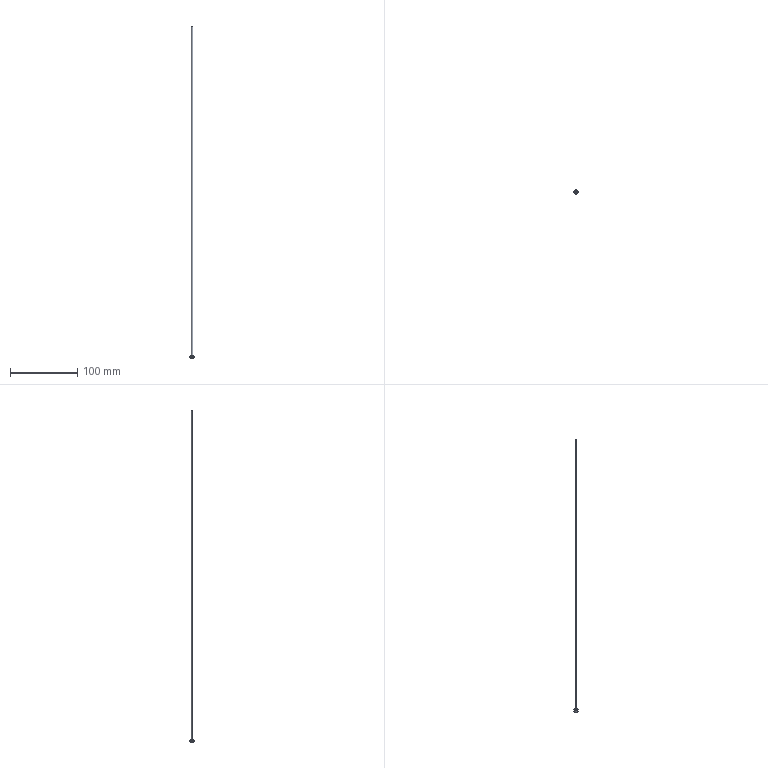Part | SolidWorks | features Chamfer 1, Extrusion 1, ICE 1 | 1 solid | 11 faces | box 6 x 6 x 493 mm | volume 1623 mm3 | cone 4 | cylinder 4 | plane 3 | commonest cylinder face diameters 2 x2 6 x2
STEP:
#1=CARTESIAN_POINT('',(-2.8,0.,-3.));
#2=VERTEX_POINT('',#1);
#3=CARTESIAN_POINT('',(2.8,0.,-3.));
#4=VERTEX_POINT('',#3);
#5=CARTESIAN_POINT('',(0.,0.,-3.));
#6=DIRECTION('',(0.,0.,-1.));
#7=DIRECTION('',(-1.,0.,0.));
#8=AXIS2_PLACEMENT_3D('',#5,#6,#7);
#9=CIRCLE('',#8,2.8);
#10=EDGE_CURVE('',#2,#4,#9,.T.);
#11=ORIENTED_EDGE('',*,*,#10,.F.);
#12=CARTESIAN_POINT('',(-3.,0.,-2.8));
#13=VERTEX_POINT('',#12);
#14=CARTESIAN_POINT('',(-2.8,0.,-3.));
#15=DIRECTION('',(-0.7071,0.,0.7071));
#16=VECTOR('',#15,1000.);
#17=LINE('',#14,#16);
#18=EDGE_CURVE('',#2,#13,#17,.T.);
#19=ORIENTED_EDGE('',*,*,#18,.T.);
#20=CARTESIAN_POINT('',(3.,0.,-2.8));
#21=VERTEX_POINT('',#20);
#22=CARTESIAN_POINT('',(0.,0.,-2.8));
#23=DIRECTION('',(0.,0.,1.));
#24=DIRECTION('',(-1.,0.,0.));
#25=AXIS2_PLACEMENT_3D('',#22,#23,#24);
#26=CIRCLE('',#25,3.);
#27=EDGE_CURVE('',#21,#13,#26,.T.);
#28=ORIENTED_EDGE('',*,*,#27,.F.);
#29=CARTESIAN_POINT('',(2.8,0.,-3.));
#30=DIRECTION('',(0.7071,0.,0.7071));
#31=VECTOR('',#30,1000.);
#32=LINE('',#29,#31);
#33=EDGE_CURVE('',#4,#21,#32,.T.);
#34=ORIENTED_EDGE('',*,*,#33,.F.);
#35=EDGE_LOOP('',(#11,#19,#28,#34));
#36=FACE_OUTER_BOUND('',#35,.T.);
#37=CARTESIAN_POINT('',(0.,0.,-3.));
#38=DIRECTION('',(0.,0.,1.));
#39=DIRECTION('',(1.,0.,0.));
#40=AXIS2_PLACEMENT_3D('',#37,#38,#39);
#41=CONICAL_SURFACE('',#40,2.8,0.7854);
#42=ADVANCED_FACE('',(#36),#41,.T.);
#43=CARTESIAN_POINT('',(2.8,0.,0.));
#44=VERTEX_POINT('',#43);
#45=CARTESIAN_POINT('',(-2.8,0.,0.));
#46=VERTEX_POINT('',#45);
#47=CARTESIAN_POINT('',(0.,0.,0.));
#48=DIRECTION('',(0.,0.,1.));
#49=DIRECTION('',(-1.,0.,0.));
#50=AXIS2_PLACEMENT_3D('',#47,#48,#49);
#51=CIRCLE('',#50,2.8);
#52=EDGE_CURVE('',#44,#46,#51,.T.);
#53=ORIENTED_EDGE('',*,*,#52,.F.);
#54=CARTESIAN_POINT('',(3.,0.,-0.2));
#55=VERTEX_POINT('',#54);
#56=CARTESIAN_POINT('',(3.,0.,-0.2));
#57=DIRECTION('',(0.7071,0.,-0.7071));
#58=VECTOR('',#57,1000.);
#59=LINE('',#56,#58);
#60=EDGE_CURVE('',#44,#55,#59,.T.);
#61=ORIENTED_EDGE('',*,*,#60,.T.);
#62=CARTESIAN_POINT('',(-3.,0.,-0.2));
#63=VERTEX_POINT('',#62);
#64=CARTESIAN_POINT('',(0.,0.,-0.2));
#65=DIRECTION('',(0.,0.,-1.));
#66=DIRECTION('',(-1.,0.,0.));
#67=AXIS2_PLACEMENT_3D('',#64,#65,#66);
#68=CIRCLE('',#67,3.);
#69=EDGE_CURVE('',#63,#55,#68,.T.);
#70=ORIENTED_EDGE('',*,*,#69,.F.);
#71=CARTESIAN_POINT('',(-3.,0.,-0.2));
#72=DIRECTION('',(-0.7071,0.,-0.7071));
#73=VECTOR('',#72,1000.);
#74=LINE('',#71,#73);
#75=EDGE_CURVE('',#46,#63,#74,.T.);
#76=ORIENTED_EDGE('',*,*,#75,.F.);
#77=EDGE_LOOP('',(#53,#61,#70,#76));
#78=FACE_OUTER_BOUND('',#77,.T.);
#79=CARTESIAN_POINT('',(0.,0.,-0.2));
#80=DIRECTION('',(0.,0.,-1.));
#81=DIRECTION('',(-1.,0.,0.));
#82=AXIS2_PLACEMENT_3D('',#79,#80,#81);
#83=CONICAL_SURFACE('',#82,3.,0.7854);
#84=ADVANCED_FACE('',(#78),#83,.T.);
#85=ORIENTED_EDGE('',*,*,#27,.T.);
#86=CARTESIAN_POINT('',(-3.,0.,-3.));
#87=DIRECTION('',(0.,0.,1.));
#88=VECTOR('',#87,1000.);
#89=LINE('',#86,#88);
#90=EDGE_CURVE('',#13,#63,#89,.T.);
#91=ORIENTED_EDGE('',*,*,#90,.T.);
#92=ORIENTED_EDGE('',*,*,#69,.T.);
#93=CARTESIAN_POINT('',(3.,0.,-3.));
#94=DIRECTION('',(0.,0.,1.));
#95=VECTOR('',#94,1000.);
#96=LINE('',#93,#95);
#97=EDGE_CURVE('',#21,#55,#96,.T.);
#98=ORIENTED_EDGE('',*,*,#97,.F.);
#99=EDGE_LOOP('',(#85,#91,#92,#98));
#100=FACE_OUTER_BOUND('',#99,.T.);
#101=CARTESIAN_POINT('',(0.,0.,-3.));
#102=DIRECTION('',(0.,0.,1.));
#103=DIRECTION('',(1.,0.,0.));
#104=AXIS2_PLACEMENT_3D('',#101,#102,#103);
#105=CYLINDRICAL_SURFACE('',#104,3.);
#106=ADVANCED_FACE('',(#100),#105,.T.);
#107=CARTESIAN_POINT('',(1.,0.,490.));
#108=VERTEX_POINT('',#107);
#109=CARTESIAN_POINT('',(-1.,0.,490.));
#110=VERTEX_POINT('',#109);
#111=CARTESIAN_POINT('',(0.,0.,490.));
#112=DIRECTION('',(0.,0.,1.));
#113=DIRECTION('',(1.,0.,0.));
#114=AXIS2_PLACEMENT_3D('',#111,#112,#113);
#115=CIRCLE('',#114,1.);
#116=EDGE_CURVE('',#108,#110,#115,.T.);
#117=ORIENTED_EDGE('',*,*,#116,.F.);
#118=CARTESIAN_POINT('',(1.,0.,0.));
#119=VERTEX_POINT('',#118);
#120=CARTESIAN_POINT('',(1.,0.,490.));
#121=DIRECTION('',(0.,0.,-1.));
#122=VECTOR('',#121,1000.);
#123=LINE('',#120,#122);
#124=EDGE_CURVE('',#108,#119,#123,.T.);
#125=ORIENTED_EDGE('',*,*,#124,.T.);
#126=CARTESIAN_POINT('',(-1.,0.,0.));
#127=VERTEX_POINT('',#126);
#128=CARTESIAN_POINT('',(0.,0.,0.));
#129=DIRECTION('',(0.,0.,1.));
#130=DIRECTION('',(1.,0.,0.));
#131=AXIS2_PLACEMENT_3D('',#128,#129,#130);
#132=CIRCLE('',#131,1.);
#133=EDGE_CURVE('',#119,#127,#132,.T.);
#134=ORIENTED_EDGE('',*,*,#133,.T.);
#135=CARTESIAN_POINT('',(-1.,0.,490.));
#136=DIRECTION('',(0.,0.,-1.));
#137=VECTOR('',#136,1000.);
#138=LINE('',#135,#137);
#139=EDGE_CURVE('',#110,#127,#138,.T.);
#140=ORIENTED_EDGE('',*,*,#139,.F.);
#141=EDGE_LOOP('',(#117,#125,#134,#140));
#142=FACE_OUTER_BOUND('',#141,.T.);
#143=CARTESIAN_POINT('',(0.,0.,490.));
#144=DIRECTION('',(0.,0.,-1.));
#145=DIRECTION('',(-1.,0.,0.));
#146=AXIS2_PLACEMENT_3D('',#143,#144,#145);
#147=CYLINDRICAL_SURFACE('',#146,1.);
#148=ADVANCED_FACE('',(#142),#147,.T.);
#149=ORIENTED_EDGE('',*,*,#124,.F.);
#150=CARTESIAN_POINT('',(0.,0.,490.));
#151=DIRECTION('',(0.,0.,1.));
#152=DIRECTION('',(1.,0.,0.));
#153=AXIS2_PLACEMENT_3D('',#150,#151,#152);
#154=CIRCLE('',#153,1.);
#155=EDGE_CURVE('',#110,#108,#154,.T.);
#156=ORIENTED_EDGE('',*,*,#155,.F.);
#157=ORIENTED_EDGE('',*,*,#139,.T.);
#158=CARTESIAN_POINT('',(0.,0.,0.));
#159=DIRECTION('',(0.,0.,1.));
#160=DIRECTION('',(1.,0.,0.));
#161=AXIS2_PLACEMENT_3D('',#158,#159,#160);
#162=CIRCLE('',#161,1.);
#163=EDGE_CURVE('',#127,#119,#162,.T.);
#164=ORIENTED_EDGE('',*,*,#163,.T.);
#165=EDGE_LOOP('',(#149,#156,#157,#164));
#166=FACE_OUTER_BOUND('',#165,.T.);
#167=CARTESIAN_POINT('',(0.,0.,490.));
#168=DIRECTION('',(0.,0.,-1.));
#169=DIRECTION('',(-1.,0.,0.));
#170=AXIS2_PLACEMENT_3D('',#167,#168,#169);
#171=CYLINDRICAL_SURFACE('',#170,1.);
#172=ADVANCED_FACE('',(#166),#171,.T.);
#173=ORIENTED_EDGE('',*,*,#155,.T.);
#174=ORIENTED_EDGE('',*,*,#116,.T.);
#175=EDGE_LOOP('',(#173,#174));
#176=FACE_OUTER_BOUND('',#175,.T.);
#177=CARTESIAN_POINT('',(0.,0.,490.));
#178=DIRECTION('',(0.,0.,1.));
#179=DIRECTION('',(1.,0.,0.));
#180=AXIS2_PLACEMENT_3D('',#177,#178,#179);
#181=PLANE('',#180);
#182=ADVANCED_FACE('',(#176),#181,.T.);
#183=ORIENTED_EDGE('',*,*,#90,.F.);
#184=CARTESIAN_POINT('',(0.,0.,-2.8));
#185=DIRECTION('',(0.,0.,1.));
#186=DIRECTION('',(-1.,0.,0.));
#187=AXIS2_PLACEMENT_3D('',#184,#185,#186);
#188=CIRCLE('',#187,3.);
#189=EDGE_CURVE('',#13,#21,#188,.T.);
#190=ORIENTED_EDGE('',*,*,#189,.T.);
#191=ORIENTED_EDGE('',*,*,#97,.T.);
#192=CARTESIAN_POINT('',(0.,0.,-0.2));
#193=DIRECTION('',(0.,0.,-1.));
#194=DIRECTION('',(-1.,0.,0.));
#195=AXIS2_PLACEMENT_3D('',#192,#193,#194);
#196=CIRCLE('',#195,3.);
#197=EDGE_CURVE('',#55,#63,#196,.T.);
#198=ORIENTED_EDGE('',*,*,#197,.T.);
#199=EDGE_LOOP('',(#183,#190,#191,#198));
#200=FACE_OUTER_BOUND('',#199,.T.);
#201=CARTESIAN_POINT('',(0.,0.,-3.));
#202=DIRECTION('',(0.,0.,1.));
#203=DIRECTION('',(1.,0.,0.));
#204=AXIS2_PLACEMENT_3D('',#201,#202,#203);
#205=CYLINDRICAL_SURFACE('',#204,3.);
#206=ADVANCED_FACE('',(#200),#205,.T.);
#207=CARTESIAN_POINT('',(0.,0.,-3.));
#208=DIRECTION('',(0.,0.,-1.));
#209=DIRECTION('',(-1.,0.,0.));
#210=AXIS2_PLACEMENT_3D('',#207,#208,#209);
#211=CIRCLE('',#210,2.8);
#212=EDGE_CURVE('',#4,#2,#211,.T.);
#213=ORIENTED_EDGE('',*,*,#212,.T.);
#214=ORIENTED_EDGE('',*,*,#10,.T.);
#215=EDGE_LOOP('',(#213,#214));
#216=FACE_OUTER_BOUND('',#215,.T.);
#217=CARTESIAN_POINT('',(0.,0.,-3.));
#218=DIRECTION('',(0.,0.,-1.));
#219=DIRECTION('',(-1.,0.,0.));
#220=AXIS2_PLACEMENT_3D('',#217,#218,#219);
#221=PLANE('',#220);
#222=ADVANCED_FACE('',(#216),#221,.T.);
#223=CARTESIAN_POINT('',(0.,0.,0.));
#224=DIRECTION('',(0.,0.,1.));
#225=DIRECTION('',(-1.,0.,0.));
#226=AXIS2_PLACEMENT_3D('',#223,#224,#225);
#227=CIRCLE('',#226,2.8);
#228=EDGE_CURVE('',#46,#44,#227,.T.);
#229=ORIENTED_EDGE('',*,*,#228,.T.);
#230=ORIENTED_EDGE('',*,*,#52,.T.);
#231=EDGE_LOOP('',(#229,#230));
#232=FACE_OUTER_BOUND('',#231,.T.);
#233=ORIENTED_EDGE('',*,*,#163,.F.);
#234=ORIENTED_EDGE('',*,*,#133,.F.);
#235=EDGE_LOOP('',(#233,#234));
#236=FACE_BOUND('',#235,.T.);
#237=CARTESIAN_POINT('',(0.,0.,0.));
#238=DIRECTION('',(0.,0.,-1.));
#239=DIRECTION('',(-1.,0.,0.));
#240=AXIS2_PLACEMENT_3D('',#237,#238,#239);
#241=PLANE('',#240);
#242=ADVANCED_FACE('',(#232,#236),#241,.F.);
#243=ORIENTED_EDGE('',*,*,#60,.F.);
#244=ORIENTED_EDGE('',*,*,#228,.F.);
#245=ORIENTED_EDGE('',*,*,#75,.T.);
#246=ORIENTED_EDGE('',*,*,#197,.F.);
#247=EDGE_LOOP('',(#243,#244,#245,#246));
#248=FACE_OUTER_BOUND('',#247,.T.);
#249=CARTESIAN_POINT('',(0.,0.,-0.2));
#250=DIRECTION('',(0.,0.,-1.));
#251=DIRECTION('',(-1.,0.,0.));
#252=AXIS2_PLACEMENT_3D('',#249,#250,#251);
#253=CONICAL_SURFACE('',#252,3.,0.7854);
#254=ADVANCED_FACE('',(#248),#253,.T.);
#255=ORIENTED_EDGE('',*,*,#18,.F.);
#256=ORIENTED_EDGE('',*,*,#212,.F.);
#257=ORIENTED_EDGE('',*,*,#33,.T.);
#258=ORIENTED_EDGE('',*,*,#189,.F.);
#259=EDGE_LOOP('',(#255,#256,#257,#258));
#260=FACE_OUTER_BOUND('',#259,.T.);
#261=CARTESIAN_POINT('',(0.,0.,-3.));
#262=DIRECTION('',(0.,0.,1.));
#263=DIRECTION('',(1.,0.,0.));
#264=AXIS2_PLACEMENT_3D('',#261,#262,#263);
#265=CONICAL_SURFACE('',#264,2.8,0.7854);
#266=ADVANCED_FACE('',(#260),#265,.T.);
#267=CLOSED_SHELL('',(#42,#84,#106,#148,#172,#182,#206,#222,#242,#254,#266));
#268=MANIFOLD_SOLID_BREP('',#267);
#269=CARTESIAN_POINT('',(0.,0.,0.));
#270=DIRECTION('',(0.,0.,1.));
#271=DIRECTION('',(1.,0.,0.));
#272=AXIS2_PLACEMENT_3D('',#269,#270,#271);
#273=(LENGTH_UNIT()NAMED_UNIT(*)SI_UNIT(.MILLI.,.METRE.));
#274=UNCERTAINTY_MEASURE_WITH_UNIT(LENGTH_MEASURE(0.00001),#273,'','');
#275=(NAMED_UNIT(*)PLANE_ANGLE_UNIT()SI_UNIT($,.RADIAN.));
#276=(NAMED_UNIT(*)SI_UNIT($,.STERADIAN.)SOLID_ANGLE_UNIT());
#277=(GEOMETRIC_REPRESENTATION_CONTEXT(3)GLOBAL_UNCERTAINTY_ASSIGNED_CONTEXT((#274))GLOBAL_UNIT_ASSIGNED_CONTEXT((#273,#275,#276))REPRESENTATION_CONTEXT('',''));
#278=ADVANCED_BREP_SHAPE_REPRESENTATION('',(#268,#272),#277);